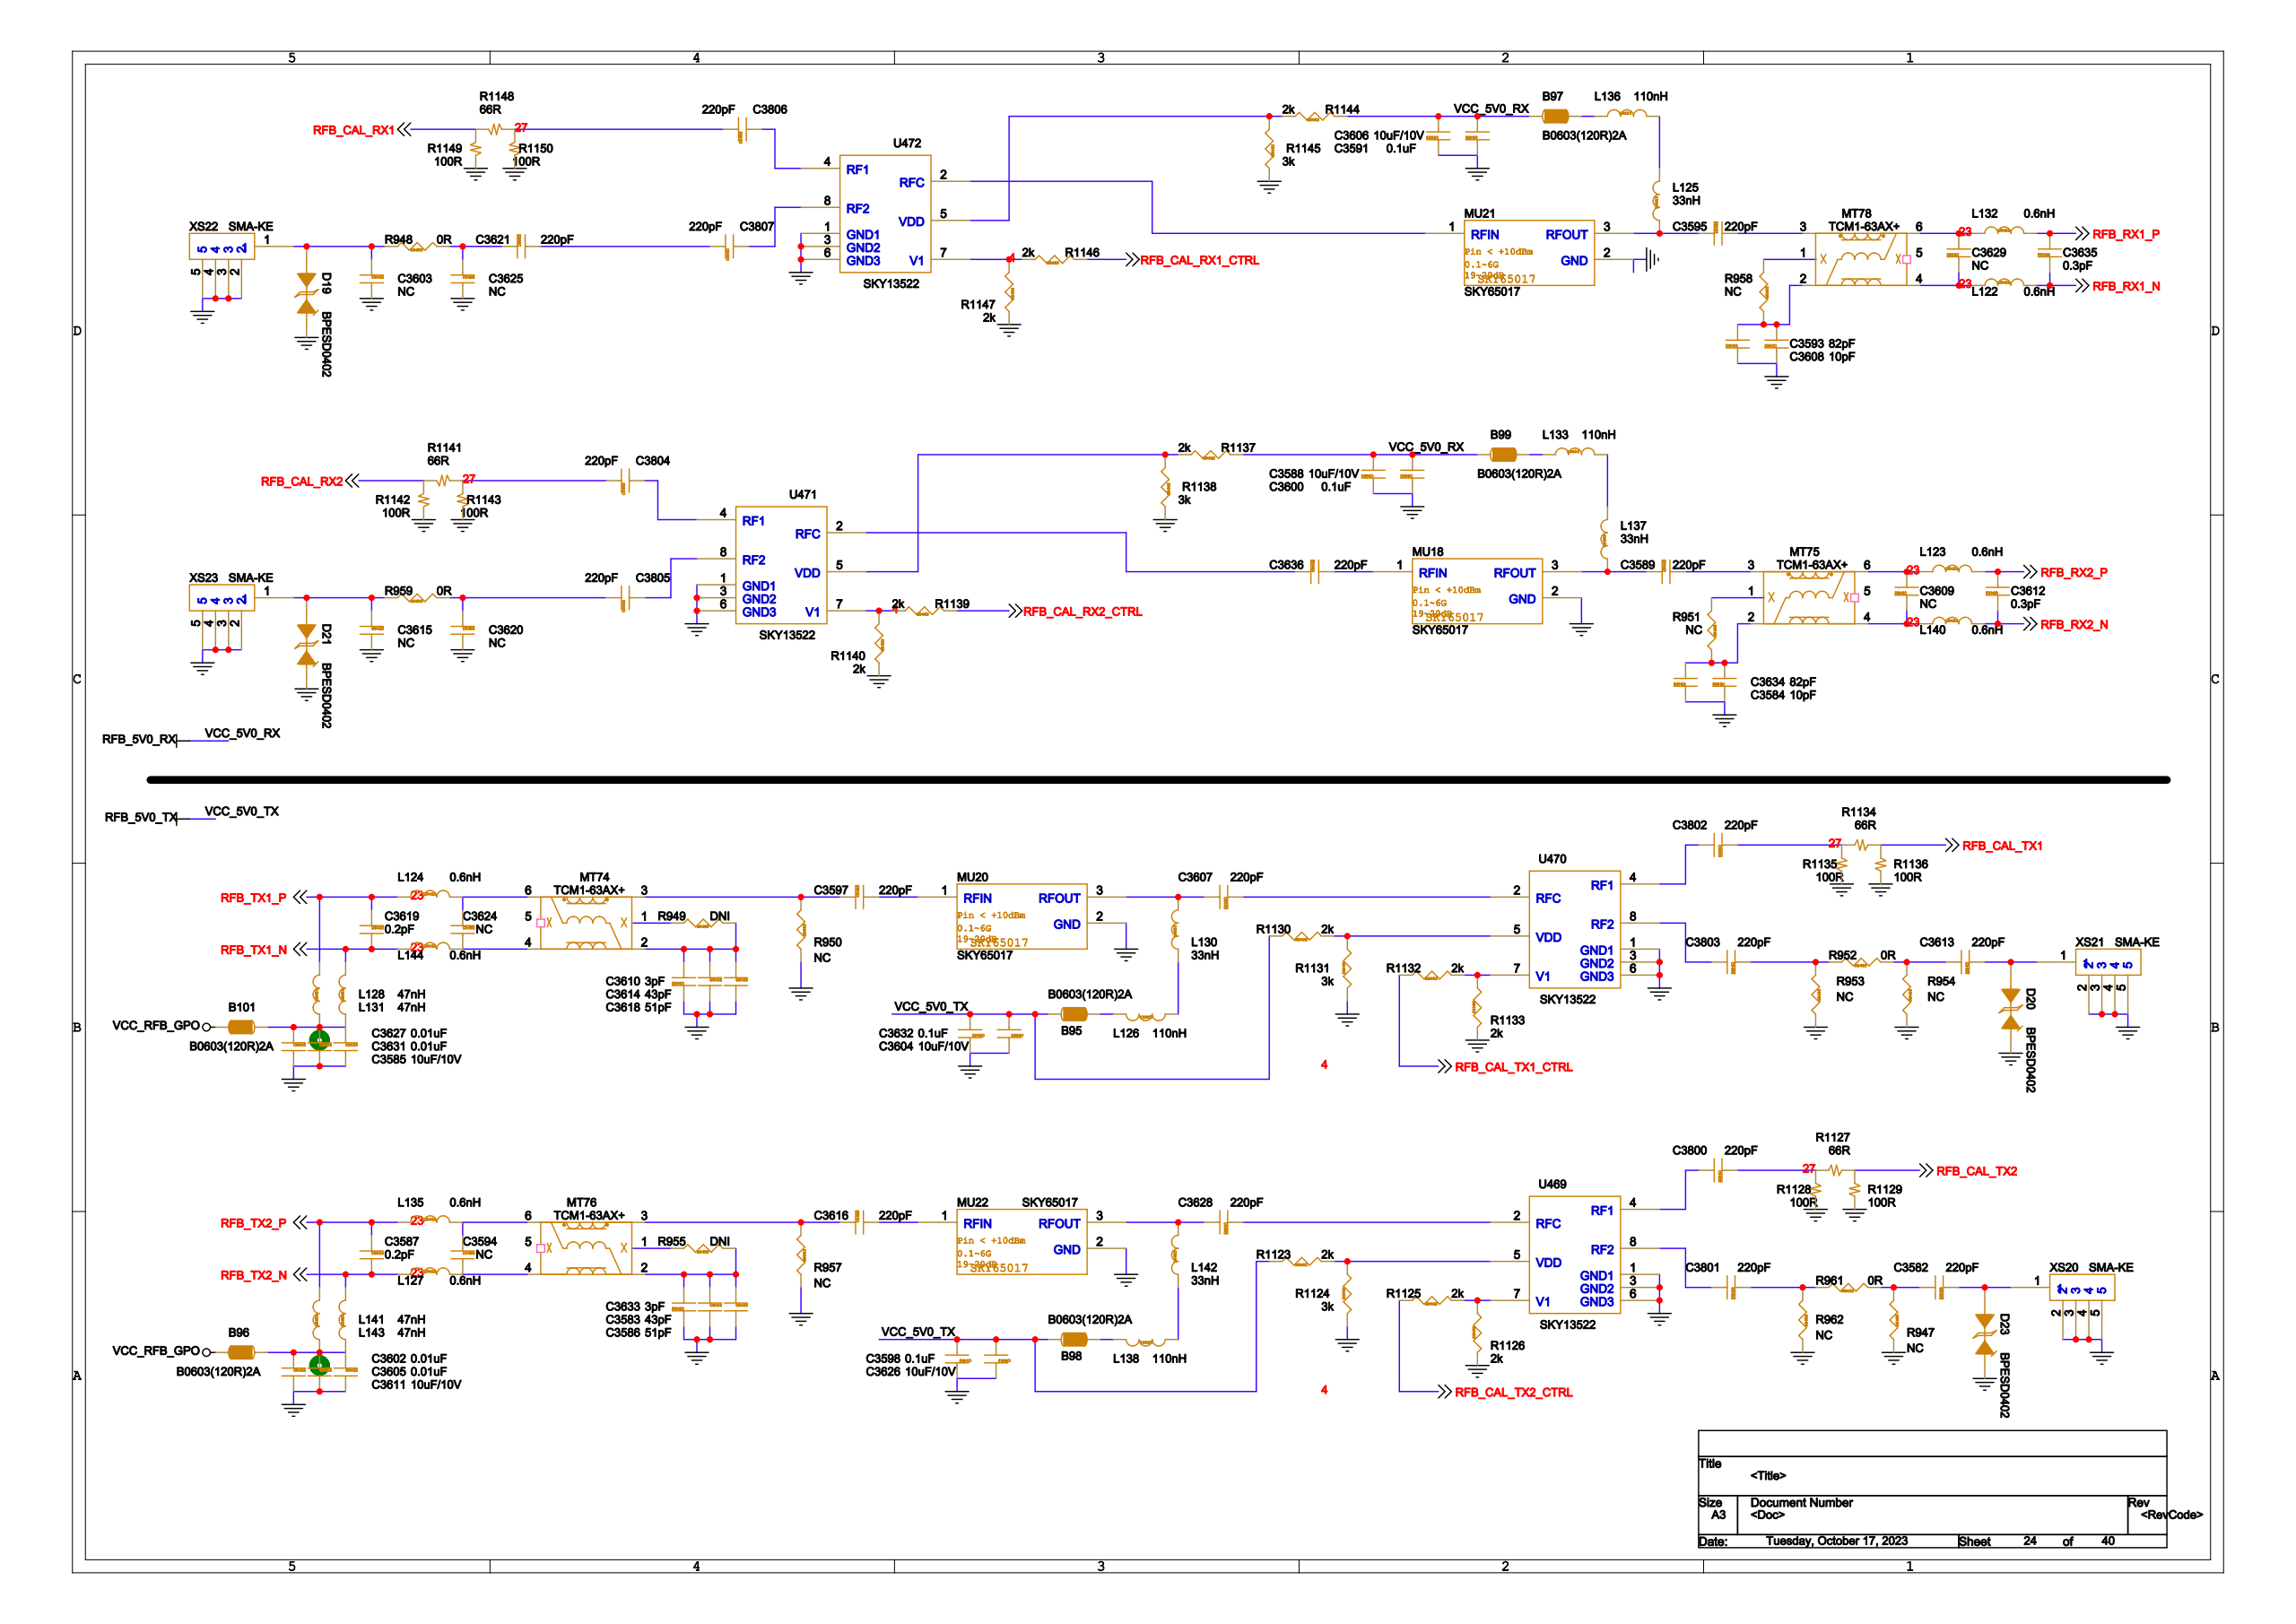Circuit board | Cadence Allegro | 1793 parts | 1223 nets | one sheet of the schematic
Parts on this sheet (reference | value | footprint):
B95 | B0603(120R)2A | B0603
B96 | B0603(120R)2A | B0603
B97 | B0603(120R)2A | B0603
B98 | B0603(120R)2A | B0603
B99 | B0603(120R)2A | B0603
B101 | B0603(120R)2A | B0603
C3582 | 220pF | C0402
C3583 | 43pF | C0402
C3584 | 10pF | C0402
C3585 | 10uF/10V | C0402
C3586 | 51pF | C0402
C3587 | 0.2pF | C0402
C3588 | 10uF/10V | C0402
C3589 | 220pF | C0402
C3591 | 0.1uF | C0402
C3593 | 82pF | C0402
C3594 | NC | C0402
C3595 | 220pF | C0402
C3597 | 220pF | C0402
C3598 | 0.1uF | C0402
C3600 | 0.1uF | C0402
C3602 | 0.01uF | C0402
C3603 | NC | C0402
C3604 | 10uF/10V | C0402
C3605 | 0.01uF | C0402
C3606 | 10uF/10V | C0402
C3607 | 220pF | C0402
C3608 | 10pF | C0402
C3609 | NC | C0402
C3610 | 3pF | C0402
C3611 | 10uF/10V | C0402
C3612 | 0.3pF | C0402
C3613 | 220pF | C0402
C3614 | 43pF | C0402
C3615 | NC | C0402
C3616 | 220pF | C0402
C3618 | 51pF | C0402
C3619 | 0.2pF | C0402
C3620 | NC | C0402
C3621 | 220pF | C0402
C3624 | NC | C0402
C3625 | NC | C0402
C3626 | 10uF/10V | C0402
C3627 | 0.01uF | C0402
C3628 | 220pF | C0402
C3629 | NC | C0402
C3631 | 0.01uF | C0402
C3632 | 0.1uF | C0402
C3633 | 3pF | C0402
C3634 | 82pF | C0402
C3635 | 0.3pF | C0402
C3636 | 220pF | C0402
C3800 | 220pF | C0402
C3801 | 220pF | C0402
C3802 | 220pF | C0402
C3803 | 220pF | C0402
C3804 | 220pF | C0402
C3805 | 220pF | C0402
C3806 | 220pF | C0402
C3807 | 220pF | C0402
D19 | BPESD0402 | C0402
D20 | BPESD0402 | C0402
D21 | BPESD0402 | C0402
D23 | BPESD0402 | C0402
L122 | 0.6nH | L0402
L123 | 0.6nH | L0402
L124 | 0.6nH | L0402
L125 | 33nH | L0603
L126 | 110nH | L0603
L127 | 0.6nH | L0402
L128 | 47nH | L0603
L130 | 33nH | L0603
L131 | 47nH | L0603
L132 | 0.6nH | L0402
L133 | 110nH | L0603
L135 | 0.6nH | L0402
L136 | 110nH | L0603
L137 | 33nH | L0603
L138 | 110nH | L0603
L140 | 0.6nH | L0402
L141 | 47nH | L0603
L142 | 33nH | L0603
L143 | 47nH | L0603
L144 | 0.6nH | L0402
MT74 | TCM1-63AX+ | TCM1-63AX
MT75 | TCM1-63AX+ | TCM1-63AX
MT76 | TCM1-63AX+ | TCM1-63AX
MT78 | TCM1-63AX+ | TCM1-63AX
MU18 | SKY65017 | SOT89_3
MU20 | SKY65017 | SOT89_3
MU21 | SKY65017 | SOT89_3
MU22 | SKY65017 | SOT89_3
R947 | NC | R0402
R948 | 0R | R0603
R949 | DNI | R0402
R950 | NC | R0402
R951 | NC | R0402
R952 | 0R | R0402
R953 | NC | R0402
R954 | NC | R0402
R955 | DNI | R0402
R957 | NC | R0402
R958 | NC | R0402
R959 | 0R | R0603
R961 | 0R | R0402
R962 | NC | R0402
R1123 | 2k | R0402
R1124 | 3k | R0402
R1125 | 2k | R0402
R1126 | 2k | R0402
R1127 | 66R | R0402
R1128 | 100R | R0402
R1129 | 100R | R0402
R1130 | 2k | R0402
R1131 | 3k | R0402
R1132 | 2k | R0402
R1133 | 2k | R0402
R1134 | 66R | R0402
R1135 | 100R | R0402
R1136 | 100R | R0402
R1137 | 2k | R0402
R1138 | 3k | R0402
R1139 | 2k | R0402
R1140 | 2k | R0402
R1141 | 66R | R0402
R1142 | 100R | R0402
R1143 | 100R | R0402
R1144 | 2k | R0402
R1145 | 3k | R0402
R1146 | 2k | R0402
R1147 | 2k | R0402
R1148 | 66R | R0402
R1149 | 100R | R0402
R1150 | 100R | R0402
U469 | SKY13522 | TSNP-8_L1_1-W1_1-P0_40-BL
U470 | SKY13522 | TSNP-8_L1_1-W1_1-P0_40-BL
U471 | SKY13522 | TSNP-8_L1_1-W1_1-P0_40-BL
U472 | SKY13522 | TSNP-8_L1_1-W1_1-P0_40-BL
XS20 | SMA-KE | SMA-SMD_BWSMA-KE-P001
XS21 | SMA-KE | SMA-SMD_BWSMA-KE-P001
XS22 | SMA-KE | SMA-SMD_BWSMA-KE-P001
XS23 | SMA-KE | SMA-SMD_BWSMA-KE-P001
Nets of these parts (net: part-pin ...):
GND: C3583-2 C3584-1 C3585-2 C3586-2 C3588-1 C3591-1 C3593-1 C3598-1 C3600-1 C3602-2 C3603-2 C3604-1 C3605-2 C3606-1 C3608-1 C3610-1 C3611-2 C3614-2 C3615-2 C3618-2 C3620-2 C3625-2 C3626-1 C3627-2 C3631-2 C3632-1 C3633-1 C3634-1 D19-2 D20-2 D21-2 D23-2 MU18-2 MU20-2 MU21-2 MU22-2 R947-1 R950-1 R953-1 R954-1 R957-1 R962-1 R1124-2 R1126-2 R1128-1 R1129-1 R1131-2 R1133-2 R1135-1 R1136-1 R1138-2 R1140-2 R1142-1 R1143-1 R1145-2 R1147-2 R1149-1 R1150-1 U469-1 U469-3 U469-6 U470-1 U470-3 U470-6 U471-1 U471-3 U471-6 U472-1 U472-3 U472-6 XS20-2 XS20-3 XS20-4 XS20-5 XS21-2 XS21-3 XS21-4 XS21-5 XS22-2 XS22-3 XS22-4 XS22-5 XS23-2 XS23-3 XS23-4 XS23-5
N17278367: C3603-1 D19-1 R948-1 XS22-1
N17278646: C3613-1 D20-1 XS21-1
N17278423: C3615-1 D21-1 R959-1 XS23-1
N17278759: C3582-1 D23-1 XS20-1
RFB_5V0_TX: B95-1 B98-1 C3598-2 C3604-2 C3626-2 C3632-2 R1123-1 R1130-1
N18700273: R1123-2 R1124-1 U469-5
RFB_CAL_TX2_CTRL: R1125-1
N18700311: R1125-2 R1126-1 U469-7
N18702029: R1130-2 R1131-1 U470-5
RFB_CAL_TX1_CTRL: R1132-1
N18702067: R1132-2 R1133-1 U470-7
RFB_5V0_RX: B97-1 B99-1 C3588-2 C3591-2 C3600-2 C3606-2 R1137-1 R1144-1
N18704238: R1137-2 R1138-1 U471-5
RFB_CAL_RX2_CTRL: R1139-1
N18704329: R1139-2 R1140-1 U471-7
N18705253: R1144-2 R1145-1 U472-5
RFB_CAL_RX1_CTRL: R1146-1
N18705336: R1146-2 R1147-1 U472-7
N18700239: C3800-1 R1127-1 R1128-2
RFB_CAL_TX2: R1127-2 R1129-2
N18701997: C3802-1 R1134-1 R1135-2
RFB_CAL_TX1: R1134-2 R1136-2
N18704262: C3804-1 R1141-1 R1143-2
RFB_CAL_RX2: R1141-2 R1142-2
N18705261: C3806-1 R1148-1 R1150-2
RFB_CAL_RX1: R1148-2 R1149-2
N18700235: C3800-2 U469-4
N18700267: C3801-2 U469-8
N18700257: C3628-1 U469-2
N18701993: C3802-2 U470-4
N18702025: C3803-2 U470-8
N18702015: C3607-1 U470-2
N18704264: C3804-2 U471-4
N18704290: C3805-2 U471-8
N18704286: C3636-1 U471-2
N18705263: C3806-2 U472-4
N18705297: C3807-2 U472-8
N17278377: MU21-1 U472-2
N17278716: B101-1 C3585-1 C3627-1 C3631-1 L128-1 L131-1
N17278829: B96-1 C3602-1 C3605-1 C3611-1 L141-1 L143-1
N17278437: C3636-2 MU18-1
N17278439: C3589-1 L137-2 MU18-3
N17278632: C3597-2 MU20-1
N17278634: C3607-2 L130-1 MU20-3
N17278304: C3595-1 L125-2 MU21-3
N17278745: C3616-2 MU22-1
N17278747: C3628-2 L142-1 MU22-3
RFB_RX1_N: C3635-1 L122-2
RFB_RX1_P: C3635-2 L132-2
RFB_RX2_N: C3612-1 L140-2
RFB_RX2_P: C3612-2 L123-2
RFB_TX1_N: C3619-2 L131-2 L144-1
RFB_TX1_P: C3619-1 L124-1 L128-2
RFB_TX2_N: C3587-2 L127-1 L143-2
RFB_TX2_P: C3587-1 L135-1 L141-2
VCC_RFB_GPO: B96-2 B101-2
N17278714: B95-2 L126-2
N17278383: B97-2 L136-2
N17278827: B98-2 L138-2
N17278411: B99-2 L133-2
N17278737: C3594-1 L135-2 MT76-6
N17278781: C3594-2 L127-2 MT76-4
N17278548: C3609-1 L140-1 MT75-4
N17278538: C3609-2 L123-1 MT75-6
N17278431: C3620-1 C3805-1 R959-2
N17278624: C3624-1 L124-2 MT74-6
N17278668: C3624-2 L144-2 MT74-4
N17278294: C3621-1 C3625-1 R948-2
N17278514: C3629-1 L122-1 MT78-4
N17278504: C3629-2 L132-1 MT78-6
N17278751: C3801-1 R961-1 R962-2
N17278638: C3803-1 R952-1 R953-2
N18705315: C3621-2 C3807-1
N17278755: C3582-2 R947-2 R961-2
N17278536: C3589-2 MT75-3
N17278300: C3595-2 MT78-3
N17278628: C3597-1 MT74-3 R950-2
N17278642: C3613-2 R952-2 R954-2
N17278741: C3616-1 MT76-3 R957-2
N17278526: C3593-2 C3608-2 MT78-2 R958-1
N17278554: C3584-2 C3634-2 MT75-2 R951-1
N17278767: C3583-1 C3586-1 C3633-2 MT76-2 R955-2
N17278654: C3610-2 C3614-1 C3618-1 MT74-2 R949-2
N17278379: L125-1 L136-1
N17278684: L126-1 L130-2
N17278413: L133-1 L137-1
N17278797: L138-1 L142-2
N17278652: MT74-1 R949-1
N17278546: MT75-1 R951-2
N17278765: MT76-1 R955-1
N17278512: MT78-1 R958-2